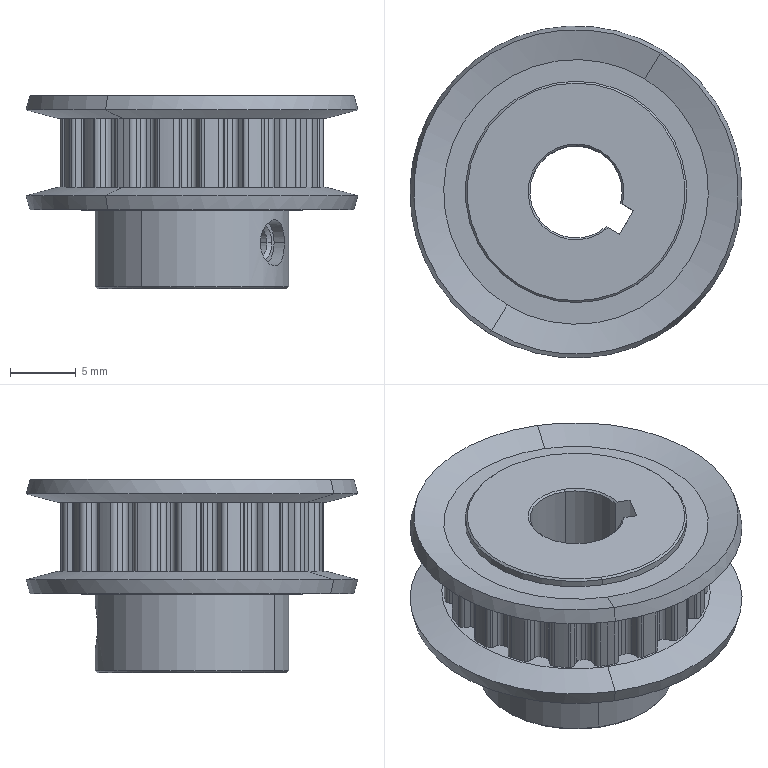Part | SolidWorks | features SplitBody 1 | 1 solid | 225 faces | box 25.2 x 25.2 x 14.7 mm | volume 3277 mm3 | cylinder 144 | plane 51 | cone 30 | commonest cylinder face diameters 0.854 x84 20.02 x19 18.06 x18 2.8 x6 2.269 x4 3.5 x4